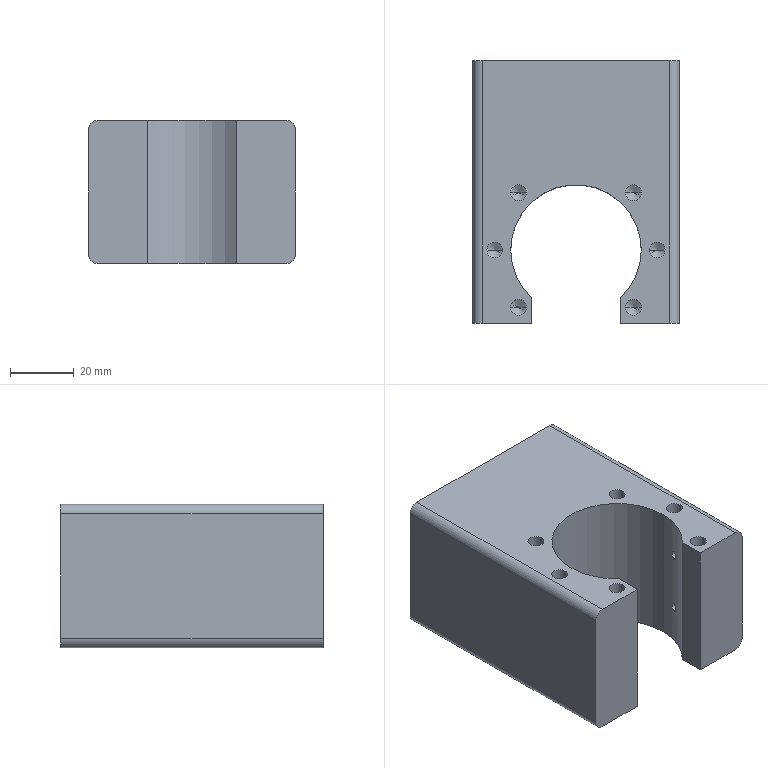Part | STEP file | 1 solid | 82 faces | box 65 x 82.5 x 45 mm | volume 171264 mm3 | cylinder 39 | cone 34 | plane 9 | commonest cylinder face diameters 5 x24 3.3 x8 6 x4 41 x3